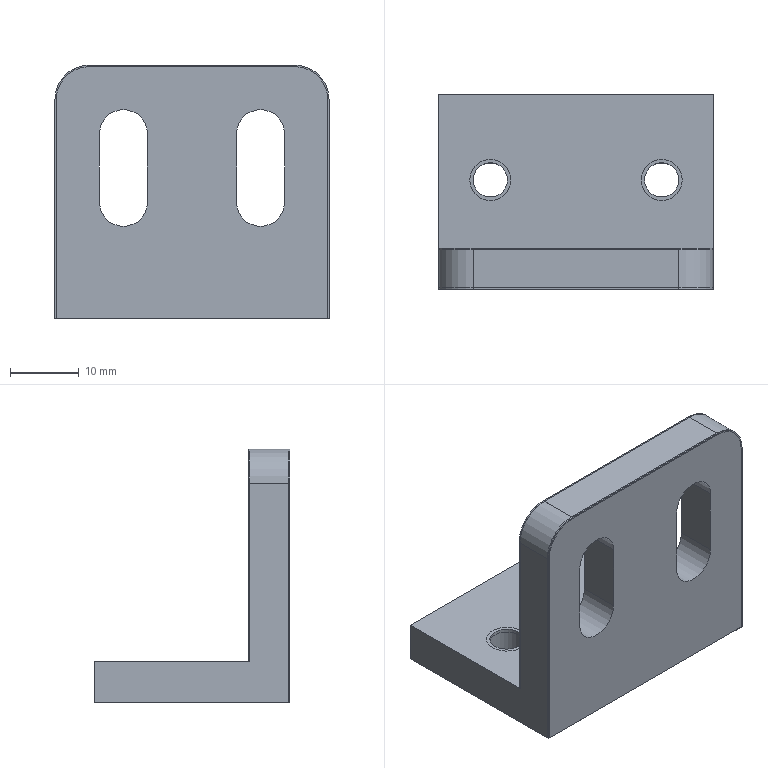NC program | NX | posted with a generic post | part box 40 x 28.5 x 37 mm
Whole program:
N10 G17 G21 G94 G90
(FLOOR_FACING , TOOL : D16CU)
N12 T01 M6
N14 G53
N16 G17 G0 G90 X33. Y11.25 B0. C0. S1500 M3
N18 G43 Z30. H1
N20 Z3.1
N22 G94 G1 Z0.1 F400.
N24 X23.
N26 X-23.
N28 X-33.
N30 Z3.1
N32 G0 Z30.
(PLANAR_MILL_COPY_1_COPY_COPY , TOOL : D16CU)
N34 X30. Y-23.85 S1300
N36 Z-37.2
N38 G1 X20. F1500.
N40 X-20.
N42 X-30.
N44 G0 Z3.
N46 X30. Y-23.6
N48 Z-37.2
N50 G1 X20.
N52 X-20.
N54 X-30.
N56 G0 Z3.
N58 X30. Y-23.35
N60 Z-37.2
N62 G1 X20.
N64 X-20.
N66 X-30.
N68 G0 Z3.
N70 X30. Y-23.1
N72 Z-37.2
N74 G1 X20.
N76 X-20.
N78 X-30.
N80 G0 Z3.
N82 X30. Y-22.85
N84 Z-37.2
N86 G1 X20.
N88 X-20.
N90 X-30.
N92 G0 Z3.
N94 X30. Y-22.6
N96 Z-37.2
N98 G1 X20.
N100 X-20.
N102 X-30.
N104 G0 Z3.
N106 X30. Y-22.35
N108 Z-37.2
N110 G1 X20.
N112 X-20.
N114 X-30.
N116 G0 Z30.
(PLANAR_MILL_COPY_1_COPY_COPY_COPY , TOOL : D16CU)
N118 X-31.1 Y-24.25
N120 Z-37.2
N122 G1 Y-14.25
N124 Y14.25
N126 Y24.25
N128 G0 Z3.
N130 X-30.85 Y-24.25
N132 Z-37.2
N134 G1 Y-14.25
N136 Y14.25
N138 Y24.25
N140 G0 Z3.
N142 X-30.6 Y-24.25
N144 Z-37.2
N146 G1 Y-14.25
N148 Y14.25
N150 Y24.25
N152 G0 Z3.
N154 X-30.35 Y-24.25
N156 Z-37.2
N158 G1 Y-14.25
N160 Y14.25
N162 Y24.25
N164 G0 Z3.
N166 X-30.1 Y-24.25
N168 Z-37.2
N170 G1 Y-14.25
N172 Y14.25
N174 Y24.25
N176 G0 Z3.
N178 X-29.85 Y-24.25
N180 Z-37.2
N182 G1 Y-14.25
N184 Y14.25
N186 Y24.25
N188 G0 Z3.
N190 X-29.6 Y-24.25
N192 Z-37.2
N194 G1 Y-14.25
N196 Y14.25
N198 Y24.25
N200 G0 Z3.
N202 X-29.35 Y-24.25
N204 Z-37.2
N206 G1 Y-14.25
N208 Y14.25
N210 Y24.25
N212 G0 Z3.
N214 X-29.1 Y-24.25
N216 Z-37.2
N218 G1 Y-14.25
N220 Y14.25
N222 Y24.25
N224 G0 Z3.
N226 X-28.85 Y-24.25
N228 Z-37.2
N230 G1 Y-14.25
N232 Y14.25
N234 Y24.25
N236 G0 Z3.
N238 X-28.6 Y-24.25
N240 Z-37.2
N242 G1 Y-14.25
N244 Y14.25
N246 Y24.25
N248 G0 Z3.
N250 X-28.35 Y-24.25
N252 Z-37.2
N254 G1 Y-14.25
N256 Y14.25
N258 Y24.25
N260 G0 Z3.
N262 X-28.1 Y-24.25
N264 Z-37.2
N266 G1 Y-14.25
N268 Y14.25
N270 Y24.25
N272 G0 Z30.
(PLANAR_MILL_COPY_1_COPY_COPY_COPY_1 , TOOL : D16CU)
N274 X-30. Y23.85
N276 Z-37.2
N278 G1 X-20.
N280 X20.
N282 X30.
N284 G0 Z3.
N286 X-30. Y23.6
N288 Z-37.2
N290 G1 X-20.
N292 X20.
N294 X30.
N296 G0 Z3.
N298 X-30. Y23.35
N300 Z-37.2
N302 G1 X-20.
N304 X20.
N306 X30.
N308 G0 Z3.
N310 X-30. Y23.1
N312 Z-37.2
N314 G1 X-20.
N316 X20.
N318 X30.
N320 G0 Z3.
N322 X-30. Y22.85
N324 Z-37.2
N326 G1 X-20.
N328 X20.
N330 X30.
N332 G0 Z3.
N334 X-30. Y22.6
N336 Z-37.2
N338 G1 X-20.
N340 X20.
N342 X30.
N344 G0 Z3.
N346 X-30. Y22.35
N348 Z-37.2
N350 G1 X-20.
N352 X20.
N354 X30.
N356 G0 Z30.
(PLANAR_MILL_COPY_1_COPY_COPY_COPY_COPY , TOOL : D16CU)
N358 X31.1 Y24.25
N360 Z-37.2
N362 G1 Y14.25
N364 Y-14.25
N366 Y-24.25
N368 G0 Z3.
N370 X30.85 Y24.25
N372 Z-37.2
N374 G1 Y14.25
N376 Y-14.25
N378 Y-24.25
N380 G0 Z3.
N382 X30.6 Y24.25
N384 Z-37.2
N386 G1 Y14.25
N388 Y-14.25
N390 Y-24.25
N392 G0 Z3.
N394 X30.35 Y24.25
N396 Z-37.2
N398 G1 Y14.25
N400 Y-14.25
N402 Y-24.25
N404 G0 Z3.
N406 X30.1 Y24.25
N408 Z-37.2
N410 G1 Y14.25
N412 Y-14.25
N414 Y-24.25
N416 G0 Z3.
N418 X29.85 Y24.25
N420 Z-37.2
N422 G1 Y14.25
N424 Y-14.25
N426 Y-24.25
N428 G0 Z3.
N430 X29.6 Y24.25
N432 Z-37.2
N434 G1 Y14.25
N436 Y-14.25
N438 Y-24.25
N440 G0 Z3.
N442 X29.35 Y24.25
N444 Z-37.2
N446 G1 Y14.25
N448 Y-14.25
N450 Y-24.25
N452 G0 Z3.
N454 X29.1 Y24.25
N456 Z-37.2
N458 G1 Y14.25
N460 Y-14.25
N462 Y-24.25
N464 G0 Z3.
N466 X28.85 Y24.25
N468 Z-37.2
N470 G1 Y14.25
N472 Y-14.25
N474 Y-24.25
N476 G0 Z3.
N478 X28.6 Y24.25
N480 Z-37.2
N482 G1 Y14.25
N484 Y-14.25
N486 Y-24.25
N488 G0 Z3.
N490 X28.35 Y24.25
N492 Z-37.2
N494 G1 Y14.25
N496 Y-14.25
N498 Y-24.25
N500 G0 Z3.
N502 X28.1 Y24.25
N504 Z-37.2
N506 G1 Y14.25
N508 Y-14.25
N510 Y-24.25
N512 G0 Z30.
(PLANAR_MILL_COPY_1_COPY_COPY_COPY_2 , TOOL : D16CU)
N514 X30. Y-22.3
N516 Z-37.2
N518 G1 X20.
N520 X-20.
N522 X-30.
N524 G0 Z30.
(PLANAR_MILL_COPY_1_COPY_COPY_COPY_1_COPY , TOOL : D16CU)
N526 Y22.3
N528 Z-37.2
N530 G1 X-20.
N532 X20.
N534 X30.
N536 G0 Z30.
(PLANAR_MILL_COPY_1_COPY_COPY_COPY_COPY_1 , TOOL : D16CU)
N538 X-28.05 Y-24.25 S700
N540 Z-37.2
N542 G1 Y-14.25 F200.
N544 Y14.25
N546 Y24.25
N548 G0 Z30.
(PLANAR_MILL_COPY_1_COPY_COPY_COPY_COPY_COPY , TOOL : D16CU)
N550 X28.05
N552 Z-37.2
N554 G1 Y14.25
N556 Y-14.25
N558 Y-24.25
N560 G0 Z30.
N562 M5
(PLANAR_MILL , TOOL : D16.)
N564 T02 M6
N566 G53
N568 G17 G0 G90 X-21.99 Y24.091 B0. C0. S1200 M3
N570 G43 Z30. H2
N572 Z-37.2
N574 G94 G3 X-20. Y22.29 R2. F400.
N576 G1 X20.
N578 G2 X28.04 Y14.25 R8.04
N580 G1 Y-14.25
N582 G2 X20. Y-22.29 R8.04
N584 G1 X-20.
N586 G2 X-28.04 Y-14.25 R8.04
N588 G1 Y14.25
N590 G2 X-20. Y22.29 R8.04
N592 G3 X-18. Y24.29 R2.
N594 G1 X-21.993 Y24.09
N596 G3 X-20. Y22.26 R2.
N598 G1 X20.
N600 G2 X28.01 Y14.25 R8.01
N602 G1 Y-14.25
N604 G2 X20. Y-22.26 R8.01
N606 G1 X-20.
N608 G2 X-28.01 Y-14.25 R8.01
N610 G1 Y14.25
N612 G2 X-20. Y22.26 R8.01
N614 G3 X-18. Y24.29 R2.
N616 G0 Z30.
(PLANAR_MILL_COPY , TOOL : D16.)
N618 X-21.99 Y24.05 S800
N620 Z-37.2
N622 G3 X-20. Y22.25 R2. F200.
N624 G1 X20.
N626 G2 X28. Y14.25 R8.
N628 G1 Y-14.25
N630 G2 X20. Y-22.25 R8.
N632 G1 X-20.
N634 G2 X-28. Y-14.25 R8.
N636 G1 Y14.25
N638 G2 X-20. Y22.25 R8.
N640 G3 X-18. Y24.25 R2.
N642 G1 X-21.99 Y24.05
N644 G3 X-20. Y22.25 R2.
N646 G1 X20.
N648 G2 X28. Y14.25 R8.
N650 G1 Y-14.25
N652 G2 X20. Y-22.25 R8.
N654 G1 X-20.
N656 G2 X-28. Y-14.25 R8.
N658 G1 Y14.25
N660 G2 X-20. Y22.25 R8.
N662 G3 X-18. Y24.25 R2.
N664 G0 Z30.
N666 M5
(PLANAR_MILL_COPY_1_COPY , TOOL : D16CU)
N668 T01 M6
N670 G53
N672 G17 G0 G90 X30. Y-22.25 B0. C0. S1500 M3
N674 G43 Z30. H1
N676 Z-30.9
N678 G94 G1 X20. F1500.
N680 X-20.
N682 X-30.
N684 G0 Z3.
N686 X30. Y-22.
N688 Z-30.9
N690 G1 X20.
N692 X-20.
N694 X-30.
N696 G0 Z3.
N698 X30. Y-21.75
N700 Z-30.9
N702 G1 X20.
N704 X-20.
N706 X-30.
N708 G0 Z3.
N710 X30. Y-21.5
N712 Z-30.9
N714 G1 X20.
N716 X-20.
N718 X-30.
N720 G0 Z3.
N722 X30. Y-21.25
N724 Z-30.9
N726 G1 X20.
N728 X-20.
N730 X-30.
N732 G0 Z3.
N734 X30. Y-21.
N736 Z-30.9
N738 G1 X20.
N740 X-20.
N742 X-30.
N744 G0 Z3.
N746 X30. Y-20.75
N748 Z-30.9
N750 G1 X20.
N752 X-20.
N754 X-30.
N756 G0 Z3.
N758 X30. Y-20.5
N760 Z-30.9
N762 G1 X20.
N764 X-20.
N766 X-30.
N768 G0 Z3.
N770 X30. Y-20.25
N772 Z-30.9
N774 G1 X20.
N776 X-20.
N778 X-30.
N780 G0 Z3.
N782 X30. Y-20.
N784 Z-30.9
N786 G1 X20.
N788 X-20.
N790 X-30.
N792 G0 Z3.
N794 X30. Y-19.75
N796 Z-30.9
N798 G1 X20.
N800 X-20.
N802 X-30.
N804 G0 Z3.
N806 X30. Y-19.5
N808 Z-30.9
N810 G1 X20.
N812 X-20.
N814 X-30.
N816 G0 Z3.
N818 X30. Y-19.25
N820 Z-30.9
N822 G1 X20.
N824 X-20.
N826 X-30.
N828 G0 Z3.
N830 X30. Y-19.
N832 Z-30.9
N834 G1 X20.
N836 X-20.
N838 X-30.
N840 G0 Z3.
N842 X30. Y-18.75
N844 Z-30.9
N846 G1 X20.
N848 X-20.
N850 X-30.
N852 G0 Z3.
N854 X30. Y-18.5
N856 Z-30.9
N858 G1 X20.
N860 X-20.
N862 X-30.
N864 G0 Z3.
N866 X30. Y-18.25
N868 Z-30.9
N870 G1 X20.
N872 X-20.
N874 X-30.
N876 G0 Z3.
N878 X30. Y-18.
N880 Z-30.9
N882 G1 X20.
N884 X-20.
N886 X-30.
N888 G0 Z3.
N890 X30. Y-17.75
N892 Z-30.9
N894 G1 X20.
N896 X-20.
N898 X-30.
N900 G0 Z3.
N902 X30. Y-17.5
N904 Z-30.9
N906 G1 X20.
N908 X-20.
N910 X-30.
N912 G0 Z3.
N914 X30. Y-17.25
N916 Z-30.9
N918 G1 X20.
N920 X-20.
N922 X-30.
N924 G0 Z3.
N926 X30. Y-17.
N928 Z-30.9
N930 G1 X20.
N932 X-20.
N934 X-30.
N936 G0 Z3.
N938 X30. Y-16.75
N940 Z-30.9
N942 G1 X20.
N944 X-20.
N946 X-30.
N948 G0 Z3.
N950 X30. Y-16.5
N952 Z-30.9
N954 G1 X20.
N956 X-20.
N958 X-30.
N960 G0 Z3.
N962 X30. Y-16.25
N964 Z-30.9
N966 G1 X20.
N968 X-20.
N970 X-30.
N972 G0 Z3.
N974 X30. Y-16.
N976 Z-30.9
N978 G1 X20.
N980 X-20.
N982 X-30.
N984 G0 Z3.
N986 X30. Y-15.75
N988 Z-30.9
N990 G1 X20.
N992 X-20.
N994 X-30.
N996 G0 Z3.
N998 X30. Y-15.5
N1000 Z-30.9
N1002 G1 X20.
N1004 X-20.
N1006 X-30.
N1008 G0 Z3.
N1010 X30. Y-15.25
N1012 Z-30.9
N1014 G1 X20.
N1016 X-20.
N1018 X-30.
N1020 G0 Z3.
N1022 X30. Y-15.
N1024 Z-30.9
N1026 G1 X20.
N1028 X-20.
N1030 X-30.
N1032 G0 Z3.
N1034 X30. Y-14.75
N1036 Z-30.9
N1038 G1 X20.
N1040 X-20.
N1042 X-30.
N1044 G0 Z3.
N1046 X30. Y-14.5
N1048 Z-30.9
N1050 G1 X20.
N1052 X-20.
N1054 X-30.
N1056 G0 Z3.
N1058 X30. Y-14.25
N1060 Z-30.9
N1062 G1 X20.
N1064 X-20.
N1066 X-30.
N1068 G0 Z3.
N1070 X30. Y-14.
N1072 Z-30.9
N1074 G1 X20.
N1076 X-20.
N1078 X-30.
N1080 G0 Z3.
N1082 X30. Y-13.75
N1084 Z-30.9
N1086 G1 X20.
N1088 X-20.
N1090 X-30.
N1092 G0 Z3.
N1094 X30. Y-13.5
N1096 Z-30.9
N1098 G1 X20.
N1100 X-20.
N1102 X-30.
N1104 G0 Z3.
N1106 X30. Y-13.25
N1108 Z-30.9
N1110 G1 X20.
N1112 X-20.
N1114 X-30.
N1116 G0 Z3.
N1118 X30. Y-13.
N1120 Z-30.9
N1122 G1 X20.
N1124 X-20.
N1126 X-30.
N1128 G0 Z3.
N1130 X30. Y-12.75
N1132 Z-30.9
N1134 G1 X20.
N1136 X-20.
N1138 X-30.
N1140 G0 Z3.
N1142 X30. Y-12.5
N1144 Z-30.9
N1146 G1 X20.
N1148 X-20.
N1150 X-30.
N1152 G0 Z3.
N1154 X30. Y-12.25
N1156 Z-30.9
N1158 G1 X20.
N1160 X-20.
N1162 X-30.
N1164 G0 Z3.
N1166 X30. Y-12.
N1168 Z-30.9
N1170 G1 X20.
N1172 X-20.
N1174 X-30.
N1176 G0 Z3.
N1178 X30. Y-11.75
N1180 Z-30.9
N1182 G1 X20.
N1184 X-20.
N1186 X-30.
N1188 G0 Z3.
N1190 X30. Y-11.5
N1192 Z-30.9
N1194 G1 X20.
N1196 X-20.
N1198 X-30.
N1200 G0 Z3.
N1202 X30. Y-11.25
N1204 Z-30.9
N1206 G1 X20.
N1208 X-20.
N1210 X-30.
N1212 G0 Z3.
N1214 X30. Y-11.
N1216 Z-30.9
N1218 G1 X20.
N1220 X-20.
N1222 X-30.
N1224 G0 Z3.
N1226 X30. Y-10.75
N1228 Z-30.9
N1230 G1 X20.
N1232 X-20.
N1234 X-30.
N1236 G0 Z3.
N1238 X30. Y-10.5
N1240 Z-30.9
N1242 G1 X20.
N1244 X-20.
N1246 X-30.
N1248 G0 Z3.
N1250 X30. Y-10.25
N1252 Z-30.9
N1254 G1 X20.
N1256 X-20.
N1258 X-30.
N1260 G0 Z3.
N1262 X30. Y-10.
N1264 Z-30.9
N1266 G1 X20.
N1268 X-20.
N1270 X-30.
N1272 G0 Z3.
N1274 X30. Y-9.75
N1276 Z-30.9
N1278 G1 X20.
N1280 X-20.
N1282 X-30.
N1284 G0 Z3.
N1286 X30. Y-9.5
N1288 Z-30.9
N1290 G1 X20.
N1292 X-20.
N1294 X-30.
N1296 G0 Z3.
N1298 X30. Y-9.25
N1300 Z-30.9
N1302 G1 X20.
N1304 X-20.
N1306 X-30.
N1308 G0 Z3.
N1310 X30. Y-9.
N1312 Z-30.9
N1314 G1 X20.
N1316 X-20.
N1318 X-30.
N1320 G0 Z3.
N1322 X30. Y-8.75
N1324 Z-30.9
N1326 G1 X20.
N1328 X-20.
N1330 X-30.
N1332 G0 Z3.
N1334 X30. Y-8.5
N1336 Z-30.9
N1338 G1 X20.
N1340 X-20.
N1342 X-30.
N1344 G0 Z3.
N1346 X30. Y-8.25
N1348 Z-30.9
N1350 G1 X20.
N1352 X-20.
N1354 X-30.
N1356 G0 Z3.
N1358 X30. Y-8.
N1360 Z-30.9
N1362 G1 X20.
N1364 X-20.
N1366 X-30.
N1368 G0 Z3.
N1370 X30. Y-7.75
N1372 Z-30.9
N1374 G1 X20.
N1376 X-20.
N1378 X-30.
N1380 G0 Z3.
N1382 X30. Y-7.5
N1384 Z-30.9
N1386 G1 X20.
N1388 X-20.
N1390 X-30.
N1392 G0 Z3.
N1394 X30. Y-7.25
N1396 Z-30.9
N1398 G1 X20.
N1400 X-20.
N1402 X-30.
N1404 G0 Z3.
N1406 X30. Y-7.
N1408 Z-30.9
N1410 G1 X20.
N1412 X-20.
N1414 X-30.
N1416 G0 Z3.
N1418 X30. Y-6.75
N1420 Z-30.9
N1422 G1 X20.
N1424 X-20.
N1426 X-30.
N1428 G0 Z3.
N1430 X30. Y-6.5
N1432 Z-30.9
N1434 G1 X20.
N1436 X-20.
N1438 X-30.
N1440 G0 Z3.
N1442 X30. Y-6.25
N1444 Z-30.9
N1446 G1 X20.
N1448 X-20.
N1450 X-30.
N1452 G0 Z3.
N1454 X30. Y-6.
N1456 Z-30.9
N1458 G1 X20.
N1460 X-20.
N1462 X-30.
N1464 G0 Z3.
N1466 X30. Y-5.75
N1468 Z-30.9
N1470 G1 X20.
N1472 X-20.
N1474 X-30.
N1476 G0 Z3.
N1478 X30. Y-5.5
N1480 Z-30.9
N1482 G1 X20.
N1484 X-20.
N1486 X-30.
N1488 G0 Z3.
N1490 X30. Y-5.25
N1492 Z-30.9
N1494 G1 X20.
N1496 X-20.
N1498 X-30.
N1500 G0 Z3.
N1502 X30. Y-5.
N1504 Z-30.9
N1506 G1 X20.
N1508 X-20.
N1510 X-30.
N1512 G0 Z3.
N1514 X30. Y-4.75
N1516 Z-30.9
N1518 G1 X20.
N1520 X-20.
N1522 X-30.
N1524 G0 Z3.
N1526 X30. Y-4.5
N1528 Z-30.9
N1530 G1 X20.
N1532 X-20.
N1534 X-30.
N1536 G0 Z3.
N1538 X30. Y-4.25
N1540 Z-30.9
N1542 G1 X20.
N1544 X-20.
N1546 X-30.
N1548 G0 Z3.
N1550 X30. Y-4.
N1552 Z-30.9
N1554 G1 X20.
N1556 X-20.
N1558 X-30.
N1560 G0 Z3.
N1562 X30. Y-3.75
N1564 Z-30.9
N1566 G1 X20.
N1568 X-20.
N1570 X-30.
N1572 G0 Z3.
N1574 X30. Y-3.5
N1576 Z-30.9
N1578 G1 X20.
N1580 X-20.
N1582 X-30.
N1584 G0 Z3.
N1586 X30. Y-3.25
N1588 Z-30.9
N1590 G1 X20.
N1592 X-20.
N1594 X-30.
N1596 G0 Z3.
N1598 X30. Y-3.
N1600 Z-30.9
N1602 G1 X20.
N1604 X-20.
N1606 X-30.
N1608 G0 Z3.
N1610 X30. Y-2.75
N1612 Z-30.9
N1614 G1 X20.
N1616 X-20.
N1618 X-30.
N1620 G0 Z3.
N1622 X30. Y-2.5
N1624 Z-30.9
N1626 G1 X20.
N1628 X-20.
N1630 X-30.
N1632 G0 Z3.
N1634 X30. Y-2.25
N1636 Z-30.9
N1638 G1 X20.
N1640 X-20.
N1642 X-30.
N1644 G0 Z3.
N1646 X30. Y-2.
N1648 Z-30.9
N1650 G1 X20.
N1652 X-20.
N1654 X-30.
N1656 G0 Z3.
N1658 X30. Y-1.75
N1660 Z-30.9
N1662 G1 X20.
N1664 X-20.
N1666 X-30.
N1668 G0 Z3.
N1670 X30. Y-1.5
N1672 Z-30.9
N1674 G1 X20.
N1676 X-20.
N1678 X-30.
N1680 G0 Z3.
N1682 X30. Y-1.25
N1684 Z-30.9
N1686 G1 X20.
N1688 X-20.
N1690 X-30.
N1692 G0 Z3.
N1694 X30. Y-1.
N1696 Z-30.9
N1698 G1 X20.
N1700 X-20.
N1702 X-30.
N1704 G0 Z3.
N1706 X30. Y-0.75
N1708 Z-30.9
N1710 G1 X20.
N1712 X-20.
N1714 X-30.
N1716 G0 Z3.
N1718 X30. Y-0.5
N1720 Z-30.9
N1722 G1 X20.
N1724 X-20.
N1726 X-30.
N1728 G0 Z3.
N1730 X30. Y-0.25
N1732 Z-30.9
N1734 G1 X20.
N1736 X-20.
N1738 X-30.
N1740 G0 Z3.
N1742 X30. Y0.
N1744 Z-30.9
N1746 G1 X20.
N1748 X-20.
N1750 X-30.
N1752 G0 Z3.
N1754 X30. Y0.25
N1756 Z-30.9
N1758 G1 X20.
N1760 X-20.
N1762 X-30.
N1764 G0 Z30.
N1766 M5
(FLOOR_FACING_COPY , TOOL : D16.)
N1768 T02 M6
N1770 G53
N1772 G17 G0 G90 X38. Y-12.65 B0. C0. S2500 M3
N1774 G43 Z30. H2
N1776 Z-28.
N1778 G94 G1 Z-31. F700.
N1780 X28.
N1782 X-28.
N1784 Y-6.225
N1786 X28.
N1788 Y0.2
N1790 X-28.
N1792 X-38.05
N1794 Z-28.
N1796 G0 Z30.
(FLOOR_FACING_COPY_1 , TOOL : D16.)
N1798 X33. Y11.25
N1800 Z3.
N1802 G1 Z0.
N1804 X23.
N1806 X-23.
N1808 X-33.
N1810 Z3.
N1812 G0 Z30.
(PLANAR_MILL_COPY_1 , TOOL : D16.)
N1814 X30. Y0.22 S1200
N1816 Z-30.9
N1818 G1 X20. F400.
N1820 X-20.
N1822 X-30.
N1824 G0 Z30.
N1826 X30. Y0.25
N1828 Z-30.9
N1830 G1 X20.
N1832 X-20.
N1834 X-30.
N1836 G0 Z30.
(PLANAR_MILL_COPY_1_COPY_1 , TOOL : D16.)
N1838 X27.071 Y4.207 S1000
N1840 Z-30.95
N1842 G1 X25.657 Y2.793 F200.
N1844 X25.457 Y2.593
N1846 G2 X19.8 Y0.25 R8.
N1848 G1 X-19.8
N1850 G2 X-25.457 Y2.593 R8.
N1852 G1 X-25.657 Y2.793
N1854 X-27.071 Y4.207
N1856 G0 Z30.
N1858 M5
(PLANAR_MILL_COPY_COPY_1_1 , TOOL : 4倒角)
N1860 T19 M6
N1862 G53
N1864 G17 G0 G90 X23.438 Y5.735 B0. C0. S4500 M3
N1866 G43 Z30. H19
N1868 Z-32.5
N1870 G41 G94 G1 X22.803 Y6.508 F800. D19
N1872 G3 X21.5 Y6.506 R1.
N1874 G1 Y-14.25
N1876 G2 X20. Y-15.75 R1.5
N1878 G1 X-20.
N1880 G2 X-21.5 Y-14.25 R1.5
N1882 G1 Y6.506
N1884 G3 X-22.803 Y6.508 R1.
N1886 G40
N1888 G1 X-23.438 Y5.735
N1890 G0 Z30.
(PLANAR_MILL_COPY_COPY_1_1_COPY , TOOL : 4倒角)
N1892 X23.485 Y6.576
N1894 Z-1.5
N1896 G41 G1 X22.5 Y6.75
N1898 X20.
N1900 X-20.
N1902 X-22.5
N1904 G40
N1906 X-23.485 Y6.576
N1908 G0 Z30.
N1910 Y15.924
N1912 Z-1.5
N1914 G41 G1 X-22.5 Y15.75
N1916 X-20.
N1918 X20.
N1920 X22.5
N1922 G40
N1924 X23.485 Y15.924
N1926 G0 Z30.
N1928 M5
(CURVE_DRIVE , TOOL : D3球刀)
N1930 T17 M6
N1932 G53
N1934 G17 G0 G90 X-21.5 Y6.75 B0. C0. S6000 M3
N1936 G43 Z30. H17
N1938 Z0.07
N1940 G94 G1 Z-5. F1000.
N1942 Y6.751 Z-5.059
N1944 Y6.755 Z-5.118
N1946 Y6.76 Z-5.176
N1948 Y6.768 Z-5.235
N1950 Y6.779 Z-5.293
N1952 Y6.791 Z-5.35
N1954 Y6.806 Z-5.407
N1956 Y6.823 Z-5.464
N1958 Y6.843 Z-5.519
N1960 Y6.864 Z-5.574
N1962 Y6.888 Z-5.628
N1964 Y6.913 Z-5.681
N1966 Y6.941 Z-5.733
N1968 Y6.971 Z-5.784
N1970 Y7.003 Z-5.833
N1972 Y7.036 Z-5.882
N1974 Y7.072 Z-5.929
N1976 Y7.109 Z-5.974
N1978 Y7.149 Z-6.018
N1980 Y7.189 Z-6.061
N1982 Y7.232 Z-6.101
N1984 Y7.276 Z-6.141
N1986 Y7.321 Z-6.178
N1988 Y7.368 Z-6.214
N1990 Y7.417 Z-6.247
N1992 Y7.466 Z-6.279
N1994 Y7.517 Z-6.309
N1996 Y7.569 Z-6.337
N1998 Y7.622 Z-6.362
N2000 Y7.676 Z-6.386
N2002 Y7.731 Z-6.407
N2004 Y7.786 Z-6.427
N2006 Y7.843 Z-6.444
N2008 Y7.9 Z-6.459
N2010 Y7.957 Z-6.471
N2012 Y8.015 Z-6.482
N2014 Y8.074 Z-6.49
N2016 Y8.132 Z-6.495
N2018 Y8.191 Z-6.499
N2020 Y8.25 Z-6.5
N2022 Y14.25
N2024 Z-6.44
N2026 X-21.499 Z-6.409
N2028 Z-6.377
N2030 Y8.25
N2032 X-21.498 Z-6.358
N2034 Z-6.344
N2036 X-21.495 Z-6.253
N2038 Y14.25
N2040 X-21.494 Z-6.234
N2042 Z-6.216
N2044 X-21.492 Z-6.188
N2046 X-21.489 Z-6.127
N2048 Y8.25
N2050 X-21.487 Z-6.092
N2052 X-21.485 Z-6.06
N2054 X-21.48 Z-6.
N2056 Y14.25
N2058 X-21.478 Z-5.967
N2060 X-21.475 Z-5.933
N2062 X-21.472 Z-5.904
N2064 X-21.471 Z-5.889
N2066 X-21.469 Z-5.874
N2068 Y8.25
N2070 X-21.463 Z-5.809
N2072 X-21.46 Z-5.777
N2074 X-21.456 Z-5.748
N2076 Y14.25
N2078 X-21.448 Z-5.684
N2080 X-21.444 Z-5.652
N2082 X-21.441 Z-5.625
N2084 X-21.44 Z-5.622
N2086 Y8.25
N2088 X-21.427 Z-5.527
N2090 X-21.424 Z-5.511
N2092 X-21.422 Z-5.496
N2094 Y14.25
N2096 X-21.403 Z-5.379
N2098 X-21.401 Z-5.371
N2100 Y8.25
N2102 X-21.398 Z-5.356
N2104 X-21.378 Z-5.248
N2106 Y14.25
N2108 X-21.375 Z-5.232
N2110 X-21.372 Z-5.217
N2112 X-21.353 Z-5.125
N2114 Y8.25
N2116 X-21.349 Z-5.109
N2118 X-21.346 Z-5.093
N2120 X-21.339 Z-5.063
N2122 X-21.325 Z-5.002
N2124 Y14.25
N2126 X-21.317 Z-4.971
N2128 X-21.31 Z-4.94
N2130 X-21.295 Z-4.88
N2132 Y8.25
N2134 X-21.287 Z-4.849
N2136 X-21.279 Z-4.818
N2138 X-21.27 Z-4.788
N2140 X-21.266 Z-4.773
N2142 X-21.262 Z-4.758
N2144 Y14.25
N2146 X-21.245 Z-4.696
N2148 X-21.236 Z-4.666
N2150 X-21.227 Z-4.637
N2152 Y8.25
N2154 X-21.209 Z-4.576
N2156 X-21.199 Z-4.545
N2158 X-21.194 Z-4.531
N2160 X-21.192 Z-4.523
N2162 X-21.19 Z-4.516
N2164 Y14.25
N2166 X-21.16 Z-4.426
N2168 X-21.155 Z-4.411
N2170 X-21.15 Z-4.396
N2172 Y8.25
N2174 X-21.111 Z-4.284
N2176 X-21.108 Z-4.277
N2178 Y14.25
N2180 X-21.103 Z-4.262
N2182 X-21.064 Z-4.159
N2184 Y8.25
N2186 X-21.058 Z-4.144
N2188 X-21.052 Z-4.13
N2190 X-21.017 Z-4.042
N2192 Y14.25
N2194 X-21.011 Z-4.027
N2196 X-21.005 Z-4.013
N2198 X-20.993 Z-3.984
N2200 X-20.968 Z-3.926
N2202 Y8.25
N2204 X-20.956 Z-3.897
N2206 X-20.943 Z-3.868
N2208 X-20.917 Z-3.811
N2210 Y14.25
N2212 X-20.904 Z-3.782
N2214 X-20.891 Z-3.753
N2216 X-20.878 Z-3.725
N2218 X-20.871 Z-3.711
N2220 X-20.864 Z-3.697
N2222 Y8.25
N2224 X-20.837 Z-3.639
N2226 X-20.823 Z-3.611
N2228 X-20.809 Z-3.583
N2230 Y14.25
N2232 X-20.78 Z-3.527
N2234 X-20.766 Z-3.499
N2236 X-20.758 Z-3.485
N2238 X-20.755 Z-3.478
N2240 X-20.751 Z-3.471
N2242 Y8.25
N2244 X-20.706 Z-3.388
N2246 X-20.699 Z-3.374
N2248 X-20.691 Z-3.36
N2250 Y14.25
N2252 X-20.633 Z-3.257
N2254 X-20.629 Z-3.25
N2256 Y8.25
N2258 X-20.621 Z-3.236
N2260 X-20.565 Z-3.142
N2262 Y14.25
N2264 X-20.557 Z-3.128
N2266 X-20.549 Z-3.115
N2268 X-20.499 Z-3.035
N2270 Y8.25
N2272 X-20.49 Z-3.021
N2274 X-20.482 Z-3.008
N2276 X-20.465 Z-2.981
N2278 X-20.431 Z-2.929
N2280 Y14.25
N2282 X-20.413 Z-2.902
N2284 X-20.396 Z-2.876
N2286 X-20.36 Z-2.824
N2288 Y8.25
N2290 X-20.343 Z-2.798
N2292 X-20.324 Z-2.772
N2294 X-20.306 Z-2.746
N2296 X-20.297 Z-2.734
N2298 X-20.288 Z-2.721
N2300 Y14.25
N2302 X-20.251 Z-2.669
N2304 X-20.233 Z-2.644
N2306 X-20.214 Z-2.619
N2308 Y8.25
N2310 X-20.176 Z-2.568
N2312 X-20.157 Z-2.543
N2314 X-20.147 Z-2.531
N2316 X-20.142 Z-2.525
N2318 X-20.138 Z-2.518
N2320 Y14.25
N2322 X-20.079 Z-2.444
N2324 X-20.069 Z-2.431
N2326 X-20.059 Z-2.419
N2328 Y8.25
N2330 X-19.984 Z-2.328
N2332 X-19.979 Z-2.322
N2334 Y14.25
N2336 X-19.969 Z-2.31
N2338 X-19.897 Z-2.226
N2340 Y8.25
N2342 X-19.887 Z-2.214
N2344 X-19.877 Z-2.203
N2346 X-19.814 Z-2.132
N2348 Y14.25
N2350 X-19.803 Z-2.12
N2352 X-19.792 Z-2.109
N2354 X-19.771 Z-2.086
N2356 X-19.728 Z-2.04
N2358 Y8.25
N2360 X-19.706 Z-2.017
N2362 X-19.684 Z-1.994
N2364 X-19.641 Z-1.949
N2366 Y14.25
N2368 X-19.618 Z-1.926
N2370 X-19.596 Z-1.904
N2372 X-19.574 Z-1.882
N2374 X-19.563 Z-1.871
N2376 X-19.551 Z-1.86
N2378 Y8.25
N2380 X-19.506 Z-1.816
N2382 X-19.483 Z-1.794
N2384 X-19.461 Z-1.772
N2386 Y14.25
N2388 X-19.415 Z-1.729
N2390 X-19.391 Z-1.708
N2392 X-19.38 Z-1.697
N2394 X-19.374 Z-1.692
N2396 X-19.368 Z-1.687
N2398 Y8.25
N2400 X-19.298 Z-1.624
N2402 X-19.286 Z-1.613
N2404 X-19.274 Z-1.603
N2406 Y14.25
N2408 X-19.184 Z-1.526
N2410 X-19.178 Z-1.521
N2412 Y8.25
N2414 X-19.166 Z-1.511
N2416 X-19.081 Z-1.441
N2418 Y14.25
N2420 X-19.069 Z-1.431
N2422 X-19.056 Z-1.421
N2424 X-18.982 Z-1.363
N2426 Y8.25
N2428 X-18.969 Z-1.353
N2430 X-18.957 Z-1.343
N2432 X-18.932 Z-1.324
N2434 X-18.882 Z-1.287
N2436 Y14.25
N2438 X-18.856 Z-1.268
N2440 X-18.831 Z-1.249
N2442 X-18.78 Z-1.212
N2444 Y8.25
N2446 X-18.754 Z-1.194
N2448 X-18.728 Z-1.176
N2450 X-18.702 Z-1.158
N2452 X-18.689 Z-1.149
N2454 X-18.676 Z-1.14
N2456 Y14.25
N2458 X-18.624 Z-1.104
N2460 X-18.598 Z-1.087
N2462 X-18.572 Z-1.07
N2464 Y8.25
N2466 X-18.519 Z-1.035
N2468 X-18.492 Z-1.018
N2470 X-18.479 Z-1.01
N2472 X-18.472 Z-1.005
N2474 X-18.466 Z-1.001
N2476 Y14.25
N2478 X-18.385 Z-0.951
N2480 X-18.372 Z-0.943
N2482 X-18.359 Z-0.935
N2484 Y8.25
N2486 X-18.257 Z-0.875
N2488 X-18.253 Z-0.873
N2490 X-18.25 Z-0.871
N2492 Y14.25
N2494 X-18.236 Z-0.863
N2496 X-18.14 Z-0.809
N2498 Y8.25
N2500 X-18.126 Z-0.801
N2502 X-18.113 Z-0.794
N2504 X-18.029 Z-0.749
N2506 Y14.25
N2508 X-18.015 Z-0.742
N2510 X-18.001 Z-0.734
N2512 X-17.973 Z-0.72
N2514 X-17.917 Z-0.692
N2516 Y8.25
N2518 X-17.889 Z-0.677
N2520 X-17.861 Z-0.663
N2522 X-17.804 Z-0.636
N2524 Y14.25
N2526 X-17.776 Z-0.623
N2528 X-17.747 Z-0.609
N2530 X-17.718 Z-0.596
N2532 X-17.704 Z-0.589
N2534 X-17.69 Z-0.583
N2536 Y8.25
N2538 X-17.632 Z-0.557
N2540 X-17.603 Z-0.544
N2542 X-17.575 Z-0.532
N2544 Y14.25
N2546 X-17.517 Z-0.507
N2548 X-17.487 Z-0.495
N2550 X-17.473 Z-0.489
N2552 X-17.466 Z-0.486
N2554 X-17.458 Z-0.483
N2556 Y8.25
N2558 X-17.371 Z-0.448
N2560 X-17.356 Z-0.442
N2562 X-17.341 Z-0.436
N2564 Y14.25
N2566 X-17.231 Z-0.395
N2568 X-17.227 Z-0.393
N2570 X-17.223 Z-0.392
N2572 Y8.25
N2574 X-17.208 Z-0.387
N2576 X-17.104 Z-0.35
N2578 Y14.25
N2580 X-17.089 Z-0.345
N2582 X-17.074 Z-0.34
N2584 X-16.985 Z-0.311
N2586 Y8.25
N2588 X-16.97 Z-0.306
N2590 X-16.955 Z-0.301
N2592 X-16.925 Z-0.292
N2594 X-16.864 Z-0.273
N2596 Y14.25
N2598 X-16.834 Z-0.264
N2600 X-16.804 Z-0.255
N2602 X-16.743 Z-0.238
N2604 Y8.25
N2606 X-16.713 Z-0.23
N2608 X-16.682 Z-0.221
N2610 X-16.652 Z-0.214
N2612 X-16.637 Z-0.21
N2614 X-16.621 Z-0.206
N2616 Y14.25
N2618 X-16.56 Z-0.19
N2620 X-16.53 Z-0.183
N2622 X-16.499 Z-0.175
N2624 Y8.25
N2626 X-16.438 Z-0.161
N2628 X-16.407 Z-0.154
N2630 X-16.391 Z-0.151
N2632 X-16.384 Z-0.149
N2634 X-16.376 Z-0.148
N2636 Y14.25
N2638 X-16.284 Z-0.128
N2640 X-16.268 Z-0.125
N2642 X-16.26 Z-0.123
N2644 X-16.253 Z-0.122
N2646 Y8.25
N2648 X-16.136 Z-0.1
N2650 X-16.129 Z-0.099
N2652 Y14.25
N2654 X-16.121 Z-0.097
N2656 X-16.113 Z-0.096
N2658 X-16.004 Z-0.078
N2660 Y8.25
N2662 X-15.997 Z-0.077
N2664 X-15.989 Z-0.076
N2666 X-15.973 Z-0.073
N2668 X-15.88 Z-0.06
N2670 Y14.25
N2672 X-15.864 Z-0.058
N2674 X-15.848 Z-0.056
N2676 X-15.817 Z-0.052
N2678 X-15.755 Z-0.044
N2680 Y8.25
N2682 X-15.739 Z-0.042
N2684 X-15.723 Z-0.04
N2686 X-15.692 Z-0.037
N2688 X-15.629 Z-0.031
N2690 Y14.25
N2692 X-15.598 Z-0.028
N2694 X-15.567 Z-0.025
N2696 X-15.535 Z-0.022
N2698 X-15.519 Z-0.021
N2700 X-15.504 Z-0.02
N2702 Y8.25
N2704 X-15.441 Z-0.015
N2706 X-15.409 Z-0.013
N2708 X-15.378 Z-0.011
N2710 Y14.25
N2712 X-15.315 Z-0.008
N2714 X-15.284 Z-0.006
N2716 X-15.252 Z-0.005
N2718 Y8.25
N2720 X-15.189 Z-0.003
N2722 X-15.126 Z-0.001
N2724 Y14.25
N2726 X-15.063 Z0.
N2728 X-15.
N2730 Y8.25
N2732 Y8.191 Z0.001
N2734 Y8.132 Z0.005
N2736 Y8.074 Z0.01
N2738 Y8.015 Z0.018
N2740 Y7.957 Z0.029
N2742 Y7.9 Z0.041
N2744 Y7.843 Z0.056
N2746 Y7.786 Z0.073
N2748 Y7.731 Z0.093
N2750 Y7.676 Z0.114
N2752 Y7.622 Z0.138
N2754 Y7.569 Z0.163
N2756 Y7.517 Z0.191
N2758 Y7.466 Z0.221
N2760 Y7.417 Z0.253
N2762 Y7.368 Z0.286
N2764 Y7.321 Z0.322
N2766 Y7.276 Z0.359
N2768 Y7.232 Z0.399
N2770 Y7.189 Z0.439
N2772 Y7.149 Z0.482
N2774 Y7.109 Z0.526
N2776 Y7.072 Z0.571
N2778 Y7.036 Z0.618
N2780 Y7.003 Z0.667
N2782 Y6.971 Z0.716
N2784 Y6.941 Z0.767
N2786 Y6.913 Z0.819
N2788 Y6.888 Z0.872
N2790 Y6.864 Z0.926
N2792 Y6.843 Z0.981
N2794 Y6.823 Z1.036
N2796 Y6.806 Z1.093
N2798 Y6.791 Z1.15
N2800 Y6.779 Z1.207
N2802 Y6.768 Z1.265
N2804 Y6.76 Z1.324
N2806 Y6.755 Z1.382
N2808 Y6.751 Z1.441
N2810 Y6.75 Z1.5
N2812 Z2.742
N2814 G0 Z30.
(CURVE_DRIVE_COPY , TOOL : D3球刀)
N2816 X21.5 Y15.75
N2818 Z0.07
N2820 G1 Z-5.
N2822 Y15.749 Z-5.059
N2824 Y15.745 Z-5.118
N2826 Y15.74 Z-5.176
N2828 Y15.732 Z-5.235
N2830 Y15.721 Z-5.293
N2832 Y15.709 Z-5.35
N2834 Y15.694 Z-5.407
N2836 Y15.677 Z-5.464
N2838 Y15.657 Z-5.519
N2840 Y15.636 Z-5.574
N2842 Y15.612 Z-5.628
N2844 Y15.587 Z-5.681
N2846 Y15.559 Z-5.733
N2848 Y15.529 Z-5.784
N2850 Y15.497 Z-5.833
N2852 Y15.464 Z-5.882
N2854 Y15.428 Z-5.929
N2856 Y15.391 Z-5.974
N2858 Y15.351 Z-6.018
N2860 Y15.311 Z-6.061
N2862 Y15.268 Z-6.101
N2864 Y15.224 Z-6.141
N2866 Y15.179 Z-6.178
N2868 Y15.132 Z-6.214
N2870 Y15.083 Z-6.247
N2872 Y15.034 Z-6.279
N2874 Y14.983 Z-6.309
N2876 Y14.931 Z-6.337
N2878 Y14.878 Z-6.362
N2880 Y14.824 Z-6.386
N2882 Y14.769 Z-6.407
N2884 Y14.714 Z-6.427
N2886 Y14.657 Z-6.444
N2888 Y14.6 Z-6.459
N2890 Y14.543 Z-6.471
N2892 Y14.485 Z-6.482
N2894 Y14.426 Z-6.49
N2896 Y14.368 Z-6.495
N2898 Y14.309 Z-6.499
N2900 Y14.25 Z-6.5
N2902 Y13.25
N2904 Y8.25
N2906 Z-6.44
N2908 X21.499 Z-6.409
N2910 Z-6.377
N2912 Y14.25
N2914 X21.498 Z-6.358
N2916 Z-6.344
N2918 X21.495 Z-6.253
N2920 Y8.25
N2922 X21.494 Z-6.234
N2924 Z-6.216
N2926 X21.492 Z-6.188
N2928 X21.489 Z-6.127
N2930 Y14.25
N2932 X21.487 Z-6.092
N2934 X21.485 Z-6.06
N2936 X21.48 Z-6.
N2938 Y8.25
N2940 X21.478 Z-5.967
N2942 X21.475 Z-5.933
N2944 X21.472 Z-5.904
N2946 X21.471 Z-5.889
N2948 X21.469 Z-5.874
N2950 Y14.25
N2952 X21.463 Z-5.809
N2954 X21.46 Z-5.777
N2956 X21.456 Z-5.748
N2958 Y8.25
N2960 X21.448 Z-5.684
N2962 X21.444 Z-5.652
N2964 X21.441 Z-5.625
N2966 X21.44 Z-5.622
N2968 Y14.25
N2970 X21.427 Z-5.527
N2972 X21.424 Z-5.511
N2974 X21.422 Z-5.496
N2976 Y8.25
N2978 X21.403 Z-5.379
N2980 X21.401 Z-5.371
N2982 Y14.25
N2984 X21.398 Z-5.356
N2986 X21.378 Z-5.248
N2988 Y8.25
N2990 X21.375 Z-5.232
N2992 X21.372 Z-5.217
N2994 X21.353 Z-5.125
N2996 Y14.25
N2998 X21.349 Z-5.109
N3000 X21.346 Z-5.093
N3002 X21.339 Z-5.063
N3004 X21.325 Z-5.002
N3006 Y8.25
N3008 X21.317 Z-4.971
N3010 X21.31 Z-4.94
N3012 X21.295 Z-4.88
N3014 Y14.25
N3016 X21.287 Z-4.849
N3018 X21.279 Z-4.818
N3020 X21.27 Z-4.788
N3022 X21.266 Z-4.773
N3024 X21.262 Z-4.758
N3026 Y8.25
N3028 X21.245 Z-4.696
N3030 X21.236 Z-4.666
N3032 X21.227 Z-4.637
N3034 Y14.25
N3036 X21.209 Z-4.576
N3038 X21.199 Z-4.545
N3040 X21.194 Z-4.531
N3042 X21.192 Z-4.523
N3044 X21.19 Z-4.516
N3046 Y8.25
N3048 X21.16 Z-4.426
N3050 X21.155 Z-4.411
N3052 X21.15 Z-4.396
N3054 Y14.25
N3056 X21.111 Z-4.284
N3058 X21.108 Z-4.277
N3060 Y8.25
N3062 X21.103 Z-4.262
N3064 X21.064 Z-4.159
N3066 Y14.25
N3068 X21.058 Z-4.144
N3070 X21.052 Z-4.13
N3072 X21.017 Z-4.042
N3074 Y8.25
N3076 X21.011 Z-4.027
N3078 X21.005 Z-4.013
N3080 X20.993 Z-3.984
N3082 X20.968 Z-3.926
N3084 Y14.25
N3086 X20.956 Z-3.897
N3088 X20.943 Z-3.868
N3090 X20.917 Z-3.811
N3092 Y8.25
N3094 X20.904 Z-3.782
N3096 X20.891 Z-3.753
N3098 X20.878 Z-3.725
N3100 X20.871 Z-3.711
N3102 X20.864 Z-3.697
N3104 Y14.25
N3106 X20.837 Z-3.639
N3108 X20.823 Z-3.611
N3110 X20.809 Z-3.583
N3112 Y8.25
N3114 X20.78 Z-3.527
N3116 X20.766 Z-3.499
N3118 X20.758 Z-3.485
N3120 X20.755 Z-3.478
N3122 X20.751 Z-3.471
N3124 Y14.25
N3126 X20.706 Z-3.388
N3128 X20.699 Z-3.374
N3130 X20.691 Z-3.36
N3132 Y8.25
N3134 X20.633 Z-3.257
N3136 X20.629 Z-3.25
N3138 Y14.25
N3140 X20.621 Z-3.236
N3142 X20.565 Z-3.142
N3144 Y8.25
N3146 X20.557 Z-3.128
N3148 X20.549 Z-3.115
N3150 X20.499 Z-3.035
N3152 Y14.25
N3154 X20.49 Z-3.021
N3156 X20.482 Z-3.008
N3158 X20.465 Z-2.981
N3160 X20.431 Z-2.929
N3162 Y8.25
N3164 X20.413 Z-2.902
N3166 X20.396 Z-2.876
N3168 X20.36 Z-2.824
N3170 Y14.25
N3172 X20.343 Z-2.798
N3174 X20.324 Z-2.772
N3176 X20.306 Z-2.746
N3178 X20.297 Z-2.734
N3180 X20.288 Z-2.721
N3182 Y8.25
N3184 X20.251 Z-2.669
N3186 X20.233 Z-2.644
N3188 X20.214 Z-2.619
N3190 Y14.25
N3192 X20.176 Z-2.568
N3194 X20.157 Z-2.543
N3196 X20.147 Z-2.531
N3198 X20.142 Z-2.525
N3200 X20.138 Z-2.518
N3202 Y8.25
N3204 X20.079 Z-2.444
N3206 X20.069 Z-2.431
N3208 X20.059 Z-2.419
N3210 Y14.25
N3212 X19.984 Z-2.328
N3214 X19.979 Z-2.322
N3216 Y8.25
N3218 X19.969 Z-2.31
N3220 X19.897 Z-2.226
N3222 Y14.25
N3224 X19.887 Z-2.214
N3226 X19.877 Z-2.203
N3228 X19.814 Z-2.132
N3230 Y8.25
N3232 X19.803 Z-2.12
N3234 X19.792 Z-2.109
N3236 X19.771 Z-2.086
N3238 X19.728 Z-2.04
N3240 Y14.25
N3242 X19.706 Z-2.017
N3244 X19.684 Z-1.994
N3246 X19.641 Z-1.949
N3248 Y8.25
N3250 X19.618 Z-1.926
N3252 X19.596 Z-1.904
N3254 X19.574 Z-1.882
N3256 X19.563 Z-1.871
N3258 X19.551 Z-1.86
N3260 Y14.25
N3262 X19.506 Z-1.816
N3264 X19.483 Z-1.794
N3266 X19.461 Z-1.772
N3268 Y8.25
N3270 X19.415 Z-1.729
N3272 X19.391 Z-1.708
N3274 X19.38 Z-1.697
N3276 X19.374 Z-1.692
N3278 X19.368 Z-1.687
N3280 Y14.25
N3282 X19.298 Z-1.624
N3284 X19.286 Z-1.613
N3286 X19.274 Z-1.603
N3288 Y8.25
N3290 X19.184 Z-1.526
N3292 X19.178 Z-1.521
N3294 Y14.25
N3296 X19.166 Z-1.511
N3298 X19.081 Z-1.441
N3300 Y8.25
N3302 X19.069 Z-1.431
N3304 X19.056 Z-1.421
N3306 X18.982 Z-1.363
N3308 Y14.25
N3310 X18.969 Z-1.353
N3312 X18.957 Z-1.343
N3314 X18.932 Z-1.324
N3316 X18.882 Z-1.287
N3318 Y8.25
N3320 X18.856 Z-1.268
N3322 X18.831 Z-1.249
N3324 X18.78 Z-1.212
N3326 Y14.25
N3328 X18.754 Z-1.194
N3330 X18.728 Z-1.176
N3332 X18.702 Z-1.158
N3334 X18.689 Z-1.149
N3336 X18.676 Z-1.14
N3338 Y8.25
N3340 X18.624 Z-1.104
N3342 X18.598 Z-1.087
N3344 X18.572 Z-1.07
N3346 Y14.25
N3348 X18.519 Z-1.035
N3350 X18.492 Z-1.018
N3352 X18.479 Z-1.01
N3354 X18.472 Z-1.005
N3356 X18.466 Z-1.001
N3358 Y8.25
N3360 X18.385 Z-0.951
N3362 X18.372 Z-0.943
N3364 X18.359 Z-0.935
N3366 Y14.25
N3368 X18.257 Z-0.875
N3370 X18.253 Z-0.873
N3372 X18.25 Z-0.871
N3374 Y8.25
N3376 X18.236 Z-0.863
N3378 X18.14 Z-0.809
N3380 Y14.25
N3382 X18.126 Z-0.801
N3384 X18.113 Z-0.794
N3386 X18.029 Z-0.749
N3388 Y8.25
N3390 X18.015 Z-0.742
N3392 X18.001 Z-0.734
N3394 X17.973 Z-0.72
N3396 X17.917 Z-0.692
N3398 Y14.25
N3400 X17.889 Z-0.677
N3402 X17.861 Z-0.663
N3404 X17.804 Z-0.636
N3406 Y8.25
N3408 X17.776 Z-0.623
N3410 X17.747 Z-0.609
N3412 X17.718 Z-0.596
N3414 X17.704 Z-0.589
N3416 X17.69 Z-0.583
N3418 Y14.25
N3420 X17.632 Z-0.557
N3422 X17.603 Z-0.544
N3424 X17.575 Z-0.532
N3426 Y8.25
N3428 X17.517 Z-0.507
N3430 X17.487 Z-0.495
N3432 X17.473 Z-0.489
N3434 X17.466 Z-0.486
N3436 X17.458 Z-0.483
N3438 Y14.25
N3440 X17.371 Z-0.448
N3442 X17.356 Z-0.442
N3444 X17.341 Z-0.436
N3446 Y8.25
N3448 X17.231 Z-0.395
N3450 X17.227 Z-0.393
N3452 X17.223 Z-0.392
N3454 Y14.25
N3456 X17.208 Z-0.387
N3458 X17.104 Z-0.35
N3460 Y8.25
N3462 X17.089 Z-0.345
N3464 X17.074 Z-0.34
N3466 X16.985 Z-0.311
N3468 Y14.25
N3470 X16.97 Z-0.306
N3472 X16.955 Z-0.301
N3474 X16.925 Z-0.292
N3476 X16.864 Z-0.273
N3478 Y8.25
N3480 X16.834 Z-0.264
N3482 X16.804 Z-0.255
N3484 X16.743 Z-0.238
N3486 Y14.25
N3488 X16.713 Z-0.23
N3490 X16.682 Z-0.221
N3492 X16.652 Z-0.214
N3494 X16.637 Z-0.21
N3496 X16.621 Z-0.206
N3498 Y8.25
N3500 X16.56 Z-0.19
N3502 X16.53 Z-0.183
N3504 X16.499 Z-0.175
N3506 Y14.25
N3508 X16.438 Z-0.161
N3510 X16.407 Z-0.154
N3512 X16.391 Z-0.151
N3514 X16.384 Z-0.149
N3516 X16.376 Z-0.148
N3518 Y8.25
N3520 X16.284 Z-0.128
N3522 X16.268 Z-0.125
N3524 X16.26 Z-0.123
N3526 X16.253 Z-0.122
N3528 Y14.25
N3530 X16.136 Z-0.1
N3532 X16.129 Z-0.099
N3534 Y8.25
N3536 X16.121 Z-0.097
N3538 X16.113 Z-0.096
N3540 X16.004 Z-0.078
N3542 Y14.25
N3544 X15.997 Z-0.077
N3546 X15.989 Z-0.076
N3548 X15.973 Z-0.073
N3550 X15.88 Z-0.06
N3552 Y8.25
N3554 X15.864 Z-0.058
N3556 X15.848 Z-0.056
N3558 X15.817 Z-0.052
N3560 X15.755 Z-0.044
N3562 Y14.25
N3564 X15.739 Z-0.042
N3566 X15.723 Z-0.04
N3568 X15.692 Z-0.037
N3570 X15.629 Z-0.031
N3572 Y8.25
N3574 X15.598 Z-0.028
N3576 X15.567 Z-0.025
N3578 X15.535 Z-0.022
N3580 X15.519 Z-0.021
N3582 X15.504 Z-0.02
N3584 Y14.25
N3586 X15.441 Z-0.015
N3588 X15.409 Z-0.013
N3590 X15.378 Z-0.011
N3592 Y8.25
N3594 X15.315 Z-0.008
N3596 X15.284 Z-0.006
N3598 X15.252 Z-0.005
N3600 Y14.25
N3602 X15.189 Z-0.003
N3604 X15.126 Z-0.001
N3606 Y8.25
N3608 X15.063 Z0.
N3610 X15.
N3612 Y14.25
N3614 Y14.309 Z0.001
N3616 Y14.368 Z0.005
N3618 Y14.426 Z0.01
N3620 Y14.485 Z0.018
N3622 Y14.543 Z0.029
N3624 Y14.6 Z0.041
N3626 Y14.657 Z0.056
N3628 Y14.714 Z0.073
N3630 Y14.769 Z0.093
N3632 Y14.824 Z0.114
N3634 Y14.878 Z0.138
N3636 Y14.931 Z0.163
N3638 Y14.983 Z0.191
N3640 Y15.034 Z0.221
N3642 Y15.083 Z0.253
N3644 Y15.132 Z0.286
N3646 Y15.179 Z0.322
N3648 Y15.224 Z0.359
N3650 Y15.268 Z0.399
N3652 Y15.311 Z0.439
N3654 Y15.351 Z0.482
N3656 Y15.391 Z0.526
N3658 Y15.428 Z0.571
N3660 Y15.464 Z0.618
N3662 Y15.497 Z0.667
N3664 Y15.529 Z0.716
N3666 Y15.559 Z0.767
N3668 Y15.587 Z0.819
N3670 Y15.612 Z0.872
N3672 Y15.636 Z0.926
N3674 Y15.657 Z0.981
N3676 Y15.677 Z1.036
N3678 Y15.694 Z1.093
N3680 Y15.709 Z1.15
N3682 Y15.721 Z1.207
N3684 Y15.732 Z1.265
N3686 Y15.74 Z1.324
N3688 Y15.745 Z1.382
N3690 Y15.749 Z1.441
N3692 Y15.75 Z1.5
N3694 Z2.742
N3696 G0 Z30.
(CURVE_DRIVE_COPY_1 , TOOL : D3球刀)
N3698 X22.603 Y7.389
N3700 Z-1.136
N3702 G1 Z-7.956 F500.
N3704 X22.026 Z-7.859
N3706 X21.53 Z-7.548
N3708 X21.191 Z-7.07
N3710 X21.061 Z-6.5
N3712 X21.059 Z-6.437
N3714 X21.053 Z-6.325
N3716 X21.044 Z-6.14
N3718 X21.031 Z-5.906
N3720 X21.015 Z-5.787
N3722 X20.995 Z-5.652
N3724 X20.971 Z-5.492
N3726 X20.944 Z-5.318
N3728 X20.913 Z-5.198
N3730 X20.879 Z-5.085
N3732 X20.841 Z-4.96
N3734 X20.8 Z-4.824
N3736 X20.755 Z-4.676
N3738 X20.706 Z-4.516
N3740 X20.655 Z-4.345
N3742 X20.599 Z-4.181
N3744 X20.541 Z-4.06
N3746 X20.479 Z-3.944
N3748 X20.414 Z-3.822
N3750 X20.345 Z-3.694
N3752 X20.273 Z-3.56
N3754 X20.198 Z-3.42
N3756 X20.12 Z-3.274
N3758 X20.039 Z-3.133
N3760 X19.955 Z-3.022
N3762 X19.868 Z-2.916
N3764 X19.778 Z-2.806
N3766 X19.685 Z-2.693
N3768 X19.589 Z-2.576
N3770 X19.491 Z-2.456
N3772 X19.389 Z-2.333
N3774 X19.286 Z-2.214
N3776 X19.179 Z-2.12
N3778 X19.07 Z-2.031
N3780 X18.959 Z-1.94
N3782 X18.845 Z-1.846
N3784 X18.729 Z-1.751
N3786 X18.61 Z-1.654
N3788 X18.49 Z-1.555
N3790 X18.367 Z-1.461
N3792 X18.242 Z-1.388
N3794 X18.116 Z-1.321
N3796 X17.987 Z-1.252
N3798 X17.857 Z-1.182
N3800 X17.725 Z-1.112
N3802 X17.591 Z-1.04
N3804 X17.456 Z-0.968
N3806 X17.319 Z-0.901
N3808 X17.181 Z-0.853
N3810 X17.042 Z-0.811
N3812 X16.901 Z-0.768
N3814 X16.759 Z-0.725
N3816 X16.616 Z-0.682
N3818 X16.473 Z-0.638
N3820 X16.328 Z-0.595
N3822 X16.182 Z-0.556
N3824 X16.036 Z-0.533
N3826 X15.889 Z-0.511
N3828 X15.742 Z-0.489
N3830 X15.594 Z-0.469
N3832 X15.446 Z-0.46
N3834 X15.297 Z-0.453
N3836 X15.149 Z-0.445
N3838 X15. Z-0.439
N3840 X5.186
N3842 X5.127
N3844 X-11.221
N3846 X-11.338
N3848 X-15.
N3850 X-15.149 Z-0.445
N3852 X-15.297 Z-0.453
N3854 X-15.446 Z-0.46
N3856 X-15.594 Z-0.469
N3858 X-15.742 Z-0.489
N3860 X-15.889 Z-0.511
N3862 X-16.036 Z-0.533
N3864 X-16.182 Z-0.556
N3866 X-16.328 Z-0.595
N3868 X-16.473 Z-0.638
N3870 X-16.616 Z-0.682
N3872 X-16.759 Z-0.725
N3874 X-16.901 Z-0.768
N3876 X-17.042 Z-0.811
N3878 X-17.181 Z-0.853
N3880 X-17.319 Z-0.901
N3882 X-17.456 Z-0.968
N3884 X-17.591 Z-1.04
N3886 X-17.725 Z-1.112
N3888 X-17.857 Z-1.182
N3890 X-17.987 Z-1.252
N3892 X-18.116 Z-1.321
N3894 X-18.242 Z-1.388
N3896 X-18.367 Z-1.461
N3898 X-18.49 Z-1.555
N3900 X-18.61 Z-1.654
N3902 X-18.729 Z-1.751
N3904 X-18.845 Z-1.846
N3906 X-18.959 Z-1.94
N3908 X-19.07 Z-2.031
N3910 X-19.179 Z-2.12
N3912 X-19.286 Z-2.214
N3914 X-19.389 Z-2.333
N3916 X-19.491 Z-2.456
N3918 X-19.589 Z-2.576
N3920 X-19.685 Z-2.693
N3922 X-19.778 Z-2.806
N3924 X-19.868 Z-2.916
N3926 X-19.955 Z-3.022
N3928 X-20.039 Z-3.133
N3930 X-20.12 Z-3.274
N3932 X-20.198 Z-3.42
N3934 X-20.273 Z-3.56
N3936 X-20.345 Z-3.694
N3938 X-20.414 Z-3.822
N3940 X-20.479 Z-3.944
N3942 X-20.541 Z-4.06
N3944 X-20.599 Z-4.181
N3946 X-20.655 Z-4.345
N3948 X-20.706 Z-4.516
N3950 X-20.755 Z-4.676
N3952 X-20.8 Z-4.824
N3954 X-20.841 Z-4.96
N3956 X-20.879 Z-5.085
N3958 X-20.913 Z-5.198
N3960 X-20.944 Z-5.318
N3962 X-20.971 Z-5.492
N3964 X-20.995 Z-5.652
N3966 X-21.015 Z-5.787
N3968 X-21.031 Z-5.906
N3970 X-21.044 Z-6.14
N3972 X-21.053 Z-6.325
N3974 X-21.059 Z-6.437
N3976 X-21.061 Z-6.5
N3978 X-21.191 Z-7.07
N3980 X-21.53 Z-7.548
N3982 X-22.026 Z-7.859
N3984 X-22.603 Z-7.956
N3986 Z-1.136
N3988 G0 Z30.
(CURVE_DRIVE_COPY_1_COPY , TOOL : D3球刀)
N3990 Y15.111
N3992 Z-1.136
N3994 G1 Z-7.956
N3996 X-22.026 Z-7.859
N3998 X-21.53 Z-7.548
N4000 X-21.191 Z-7.07
N4002 X-21.061 Z-6.5
N4004 X-21.059 Z-6.437
N4006 X-21.053 Z-6.325
N4008 X-21.044 Z-6.14
N4010 X-21.031 Z-5.906
N4012 X-21.015 Z-5.787
N4014 X-20.995 Z-5.652
N4016 X-20.971 Z-5.492
N4018 X-20.944 Z-5.318
N4020 X-20.913 Z-5.198
N4022 X-20.879 Z-5.085
N4024 X-20.841 Z-4.96
N4026 X-20.8 Z-4.824
N4028 X-20.755 Z-4.676
N4030 X-20.706 Z-4.516
N4032 X-20.655 Z-4.345
N4034 X-20.599 Z-4.181
N4036 X-20.541 Z-4.06
N4038 X-20.479 Z-3.944
N4040 X-20.414 Z-3.822
N4042 X-20.345 Z-3.694
N4044 X-20.273 Z-3.56
N4046 X-20.198 Z-3.42
N4048 X-20.12 Z-3.274
N4050 X-20.039 Z-3.133
N4052 X-19.955 Z-3.022
N4054 X-19.868 Z-2.916
N4056 X-19.778 Z-2.806
N4058 X-19.685 Z-2.693
N4060 X-19.589 Z-2.576
N4062 X-19.491 Z-2.456
N4064 X-19.389 Z-2.333
N4066 X-19.286 Z-2.214
N4068 X-19.179 Z-2.12
N4070 X-19.07 Z-2.031
N4072 X-18.959 Z-1.94
N4074 X-18.845 Z-1.846
N4076 X-18.729 Z-1.751
N4078 X-18.61 Z-1.654
N4080 X-18.49 Z-1.555
N4082 X-18.367 Z-1.461
N4084 X-18.242 Z-1.388
N4086 X-18.116 Z-1.321
N4088 X-17.987 Z-1.252
N4090 X-17.857 Z-1.182
N4092 X-17.725 Z-1.112
N4094 X-17.591 Z-1.04
N4096 X-17.456 Z-0.968
N4098 X-17.319 Z-0.901
N4100 X-17.181 Z-0.853
N4102 X-17.042 Z-0.811
N4104 X-16.901 Z-0.768
N4106 X-16.759 Z-0.725
N4108 X-16.616 Z-0.682
N4110 X-16.473 Z-0.638
N4112 X-16.328 Z-0.595
N4114 X-16.182 Z-0.556
N4116 X-16.036 Z-0.533
N4118 X-15.889 Z-0.511
N4120 X-15.742 Z-0.489
N4122 X-15.594 Z-0.469
N4124 X-15.446 Z-0.46
N4126 X-15.297 Z-0.453
N4128 X-15.149 Z-0.445
N4130 X-15. Z-0.439
N4132 X-14.619
N4134 X-14.531
N4136 X-14.473
N4138 X-8.057
N4140 X-8.027
N4142 X-7.969
N4144 X-3.604
N4146 X-3.516
N4148 X-3.398
N4150 X-3.311
N4152 X-3.223
N4154 X-3.135
N4156 X-3.018
N4158 X-2.93
N4160 X-2.813
N4162 X-2.695
N4164 X-2.637
N4166 X-2.49
N4168 X-2.432
N4170 X-1.846
N4172 X-1.787
N4174 X-1.641
N4176 X-1.553
N4178 X-1.494
N4180 X-1.113
N4182 X-1.025
N4184 X-0.938
N4186 X-0.85
N4188 X-0.791
N4190 X-0.234
N4192 X-0.146
N4194 X-0.117
N4196 X-0.059
N4198 X3.105
N4200 X3.135
N4202 X3.193
N4204 X3.252
N4206 X3.281
N4208 X3.369
N4210 X3.428
N4212 X3.516
N4214 X3.662
N4216 X3.691
N4218 X8.73
N4220 X9.111
N4222 X9.17
N4224 X15.
N4226 X15.149 Z-0.445
N4228 X15.297 Z-0.453
N4230 X15.446 Z-0.46
N4232 X15.594 Z-0.469
N4234 X15.742 Z-0.489
N4236 X15.889 Z-0.511
N4238 X16.036 Z-0.533
N4240 X16.182 Z-0.556
N4242 X16.328 Z-0.595
N4244 X16.473 Z-0.638
N4246 X16.616 Z-0.682
N4248 X16.759 Z-0.725
N4250 X16.901 Z-0.768
N4252 X17.042 Z-0.811
N4254 X17.181 Z-0.853
N4256 X17.319 Z-0.901
N4258 X17.456 Z-0.968
N4260 X17.591 Z-1.04
N4262 X17.725 Z-1.112
N4264 X17.857 Z-1.182
N4266 X17.987 Z-1.252
N4268 X18.116 Z-1.321
N4270 X18.242 Z-1.388
N4272 X18.367 Z-1.461
N4274 X18.49 Z-1.555
N4276 X18.61 Z-1.654
N4278 X18.729 Z-1.751
N4280 X18.845 Z-1.846
N4282 X18.959 Z-1.94
N4284 X19.07 Z-2.031
N4286 X19.179 Z-2.12
N4288 X19.286 Z-2.214
N4290 X19.389 Z-2.333
N4292 X19.491 Z-2.456
N4294 X19.589 Z-2.576
N4296 X19.685 Z-2.693
N4298 X19.778 Z-2.806
N4300 X19.868 Z-2.916
N4302 X19.955 Z-3.022
N4304 X20.039 Z-3.133
N4306 X20.12 Z-3.274
N4308 X20.198 Z-3.42
N4310 X20.273 Z-3.56
N4312 X20.345 Z-3.694
N4314 X20.414 Z-3.822
N4316 X20.479 Z-3.944
N4318 X20.541 Z-4.06
N4320 X20.599 Z-4.181
N4322 X20.655 Z-4.345
N4324 X20.706 Z-4.516
N4326 X20.755 Z-4.676
N4328 X20.8 Z-4.824
N4330 X20.841 Z-4.96
N4332 X20.879 Z-5.085
N4334 X20.913 Z-5.198
N4336 X20.944 Z-5.318
N4338 X20.971 Z-5.492
N4340 X20.995 Z-5.652
N4342 X21.015 Z-5.787
N4344 X21.031 Z-5.906
N4346 X21.044 Z-6.14
N4348 X21.053 Z-6.325
N4350 X21.059 Z-6.437
N4352 X21.06 Z-6.469
N4354 X21.061 Z-6.5
N4356 X21.183 Z-7.072
N4358 X21.516 Z-7.554
N4360 X22.007 Z-7.872
N4362 X22.582 Z-7.978
N4364 Z-1.109
N4366 G0 Z30.
N4368 M5
N4370 M2